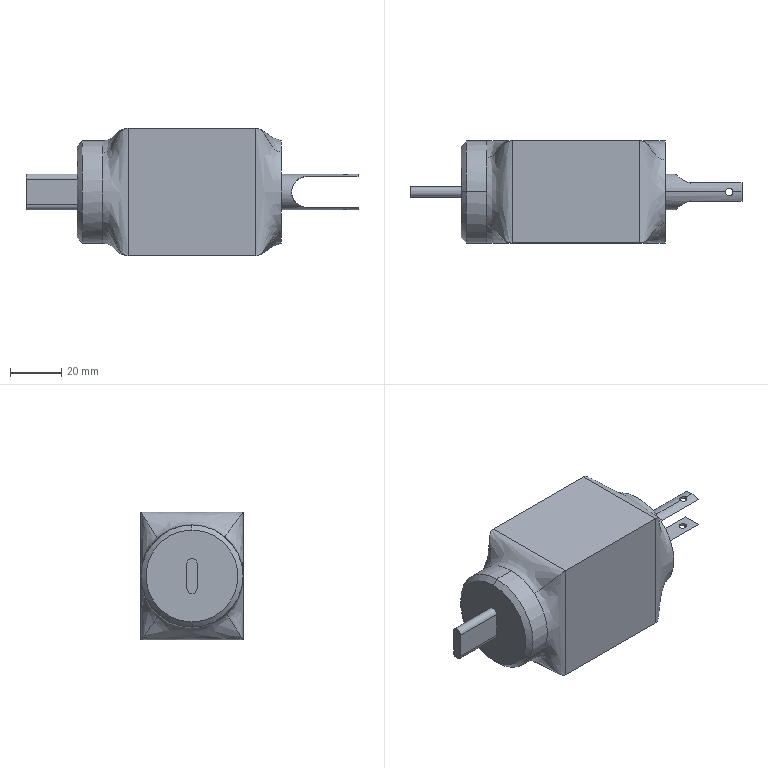Part | SolidWorks | features ICE 7, Blend 2, Chamfer 1, Extrusion 1, RefAxis 1, Revolution 1 | 1 solid | 35 faces | box 130 x 40 x 50 mm | volume 146792 mm3 | plane 13 | cylinder 12 | spline 8 | cone 2 | commonest cylinder face diameters 3 x4 4 x3 14 x2 40 x2 12 x1
STEP:
#1=CARTESIAN_POINT('',(83.5,0.,6.));
#2=VERTEX_POINT('',#1);
#3=CARTESIAN_POINT('',(86.5,0.,6.));
#4=VERTEX_POINT('',#3);
#5=CARTESIAN_POINT('',(85.,0.,6.));
#6=DIRECTION('',(0.,0.,1.));
#7=DIRECTION('',(1.,0.,0.));
#8=AXIS2_PLACEMENT_3D('',#5,#6,#7);
#9=CIRCLE('',#8,1.5);
#10=EDGE_CURVE('',#2,#4,#9,.T.);
#11=ORIENTED_EDGE('',*,*,#10,.F.);
#12=CARTESIAN_POINT('',(83.5,0.,7.));
#13=VERTEX_POINT('',#12);
#14=CARTESIAN_POINT('',(83.5,0.,-15.));
#15=DIRECTION('',(0.,0.,1.));
#16=VECTOR('',#15,1000.);
#17=LINE('',#14,#16);
#18=EDGE_CURVE('',#2,#13,#17,.T.);
#19=ORIENTED_EDGE('',*,*,#18,.T.);
#20=CARTESIAN_POINT('',(86.5,0.,7.));
#21=VERTEX_POINT('',#20);
#22=CARTESIAN_POINT('',(86.5,0.,7.));
#23=CARTESIAN_POINT('',(86.5,-0.09942,7.));
#24=CARTESIAN_POINT('',(86.49,-0.1971,6.998));
#25=CARTESIAN_POINT('',(86.452,-0.3892,6.99));
#26=CARTESIAN_POINT('',(86.423,-0.4847,6.984));
#27=CARTESIAN_POINT('',(86.348,-0.6662,6.969));
#28=CARTESIAN_POINT('',(86.301,-0.7523,6.96));
#29=CARTESIAN_POINT('',(86.193,-0.9151,6.94));
#30=CARTESIAN_POINT('',(86.129,-0.992,6.93));
#31=CARTESIAN_POINT('',(85.922,-1.199,6.898));
#32=CARTESIAN_POINT('',(85.755,-1.31,6.877));
#33=CARTESIAN_POINT('',(85.395,-1.46,6.846));
#34=CARTESIAN_POINT('',(85.197,-1.5,6.837));
#35=CARTESIAN_POINT('',(84.902,-1.5,6.837));
#36=CARTESIAN_POINT('',(84.803,-1.49,6.84));
#37=CARTESIAN_POINT('',(84.61,-1.452,6.848));
#38=CARTESIAN_POINT('',(84.516,-1.423,6.854));
#39=CARTESIAN_POINT('',(84.243,-1.31,6.877));
#40=CARTESIAN_POINT('',(84.078,-1.2,6.898));
#41=CARTESIAN_POINT('',(83.87,-0.9909,6.93));
#42=CARTESIAN_POINT('',(83.808,-0.9154,6.94));
#43=CARTESIAN_POINT('',(83.699,-0.7532,6.96));
#44=CARTESIAN_POINT('',(83.652,-0.6653,6.969));
#45=CARTESIAN_POINT('',(83.577,-0.4841,6.984));
#46=CARTESIAN_POINT('',(83.548,-0.3905,6.99));
#47=CARTESIAN_POINT('',(83.51,-0.1976,6.998));
#48=CARTESIAN_POINT('',(83.5,-0.09806,7.));
#49=CARTESIAN_POINT('',(83.5,0.,7.));
#50=B_SPLINE_CURVE_WITH_KNOTS('',3,(#22,#23,#24,#25,#26,#27,#28,#29,#30,#31,#32,#33,#34,#35,#36,#37,#38,#39,#40,#41,#42,#43,#44,#45,#46,#47,#48,#49),.UNSPECIFIED.,.F.,.F.,(4,2,2,2,2,2,2,2,2,2,2,2,2,4),(0.,0.000294,0.0005879,0.0008819,0.001176,0.001764,0.002352,0.002646,0.00294,0.003528,0.003821,0.004115,0.004409,0.004703),.UNSPECIFIED.);
#51=EDGE_CURVE('',#21,#13,#50,.T.);
#52=ORIENTED_EDGE('',*,*,#51,.F.);
#53=CARTESIAN_POINT('',(86.5,0.,-15.));
#54=DIRECTION('',(0.,0.,1.));
#55=VECTOR('',#54,1000.);
#56=LINE('',#53,#55);
#57=EDGE_CURVE('',#4,#21,#56,.T.);
#58=ORIENTED_EDGE('',*,*,#57,.F.);
#59=EDGE_LOOP('',(#11,#19,#52,#58));
#60=FACE_OUTER_BOUND('',#59,.T.);
#61=CARTESIAN_POINT('',(85.,0.,-15.));
#62=DIRECTION('',(0.,0.,1.));
#63=DIRECTION('',(1.,0.,0.));
#64=AXIS2_PLACEMENT_3D('',#61,#62,#63);
#65=CYLINDRICAL_SURFACE('',#64,1.5);
#66=ADVANCED_FACE('',(#60),#65,.F.);
#67=CARTESIAN_POINT('',(83.5,0.,-7.));
#68=VERTEX_POINT('',#67);
#69=CARTESIAN_POINT('',(86.5,0.,-7.));
#70=VERTEX_POINT('',#69);
#71=CARTESIAN_POINT('',(83.5,0.,-7.));
#72=CARTESIAN_POINT('',(83.5,-0.1961,-7.));
#73=CARTESIAN_POINT('',(83.54,-0.394,-6.991));
#74=CARTESIAN_POINT('',(83.689,-0.7552,-6.962));
#75=CARTESIAN_POINT('',(83.801,-0.9218,-6.94));
#76=CARTESIAN_POINT('',(84.008,-1.129,-6.909));
#77=CARTESIAN_POINT('',(84.085,-1.192,-6.898));
#78=CARTESIAN_POINT('',(84.247,-1.301,-6.878));
#79=CARTESIAN_POINT('',(84.333,-1.347,-6.869));
#80=CARTESIAN_POINT('',(84.606,-1.461,-6.846));
#81=CARTESIAN_POINT('',(84.801,-1.5,-6.837));
#82=CARTESIAN_POINT('',(85.098,-1.5,-6.837));
#83=CARTESIAN_POINT('',(85.196,-1.49,-6.84));
#84=CARTESIAN_POINT('',(85.388,-1.452,-6.848));
#85=CARTESIAN_POINT('',(85.484,-1.423,-6.854));
#86=CARTESIAN_POINT('',(85.756,-1.311,-6.877));
#87=CARTESIAN_POINT('',(85.922,-1.199,-6.898));
#88=CARTESIAN_POINT('',(86.198,-0.9236,-6.94));
#89=CARTESIAN_POINT('',(86.31,-0.7569,-6.961));
#90=CARTESIAN_POINT('',(86.46,-0.396,-6.991));
#91=CARTESIAN_POINT('',(86.5,-0.1988,-7.));
#92=CARTESIAN_POINT('',(86.5,0.,-7.));
#93=B_SPLINE_CURVE_WITH_KNOTS('',3,(#71,#72,#73,#74,#75,#76,#77,#78,#79,#80,#81,#82,#83,#84,#85,#86,#87,#88,#89,#90,#91,#92),.UNSPECIFIED.,.F.,.F.,(4,2,2,2,2,2,2,2,2,2,4),(0.004703,0.005291,0.005879,0.006173,0.006467,0.007054,0.007348,0.007642,0.00823,0.008818,0.009405),.UNSPECIFIED.);
#94=EDGE_CURVE('',#68,#70,#93,.T.);
#95=ORIENTED_EDGE('',*,*,#94,.F.);
#96=CARTESIAN_POINT('',(83.5,0.,-6.));
#97=VERTEX_POINT('',#96);
#98=CARTESIAN_POINT('',(83.5,0.,-15.));
#99=DIRECTION('',(0.,0.,1.));
#100=VECTOR('',#99,1000.);
#101=LINE('',#98,#100);
#102=EDGE_CURVE('',#68,#97,#101,.T.);
#103=ORIENTED_EDGE('',*,*,#102,.T.);
#104=CARTESIAN_POINT('',(86.5,0.,-6.));
#105=VERTEX_POINT('',#104);
#106=CARTESIAN_POINT('',(85.,0.,-6.));
#107=DIRECTION('',(0.,0.,-1.));
#108=DIRECTION('',(-1.,0.,0.));
#109=AXIS2_PLACEMENT_3D('',#106,#107,#108);
#110=CIRCLE('',#109,1.5);
#111=EDGE_CURVE('',#105,#97,#110,.T.);
#112=ORIENTED_EDGE('',*,*,#111,.F.);
#113=CARTESIAN_POINT('',(86.5,0.,-15.));
#114=DIRECTION('',(0.,0.,1.));
#115=VECTOR('',#114,1000.);
#116=LINE('',#113,#115);
#117=EDGE_CURVE('',#70,#105,#116,.T.);
#118=ORIENTED_EDGE('',*,*,#117,.F.);
#119=EDGE_LOOP('',(#95,#103,#112,#118));
#120=FACE_OUTER_BOUND('',#119,.T.);
#121=CARTESIAN_POINT('',(85.,0.,-15.));
#122=DIRECTION('',(0.,0.,1.));
#123=DIRECTION('',(1.,0.,0.));
#124=AXIS2_PLACEMENT_3D('',#121,#122,#123);
#125=CYLINDRICAL_SURFACE('',#124,1.5);
#126=ADVANCED_FACE('',(#120),#125,.F.);
#127=CARTESIAN_POINT('',(90.,0.,-7.));
#128=VERTEX_POINT('',#127);
#129=CARTESIAN_POINT('',(90.,3.606,-6.));
#130=VERTEX_POINT('',#129);
#131=CARTESIAN_POINT('',(90.,0.,0.));
#132=DIRECTION('',(1.,0.,0.));
#133=DIRECTION('',(0.,0.,-1.));
#134=AXIS2_PLACEMENT_3D('',#131,#132,#133);
#135=CIRCLE('',#134,7.);
#136=EDGE_CURVE('',#128,#130,#135,.T.);
#137=ORIENTED_EDGE('',*,*,#136,.F.);
#138=CARTESIAN_POINT('',(90.,0.,-7.));
#139=DIRECTION('',(-1.,0.,0.));
#140=VECTOR('',#139,1000.);
#141=LINE('',#138,#140);
#142=EDGE_CURVE('',#128,#70,#141,.T.);
#143=ORIENTED_EDGE('',*,*,#142,.T.);
#144=CARTESIAN_POINT('',(86.5,0.,-7.));
#145=CARTESIAN_POINT('',(86.5,0.09942,-7.));
#146=CARTESIAN_POINT('',(86.49,0.1971,-6.998));
#147=CARTESIAN_POINT('',(86.452,0.3892,-6.99));
#148=CARTESIAN_POINT('',(86.423,0.4847,-6.984));
#149=CARTESIAN_POINT('',(86.348,0.6662,-6.969));
#150=CARTESIAN_POINT('',(86.301,0.7523,-6.96));
#151=CARTESIAN_POINT('',(86.193,0.9151,-6.94));
#152=CARTESIAN_POINT('',(86.129,0.992,-6.93));
#153=CARTESIAN_POINT('',(85.922,1.199,-6.898));
#154=CARTESIAN_POINT('',(85.755,1.31,-6.877));
#155=CARTESIAN_POINT('',(85.395,1.46,-6.846));
#156=CARTESIAN_POINT('',(85.197,1.5,-6.837));
#157=CARTESIAN_POINT('',(84.902,1.5,-6.837));
#158=CARTESIAN_POINT('',(84.803,1.49,-6.84));
#159=CARTESIAN_POINT('',(84.61,1.452,-6.848));
#160=CARTESIAN_POINT('',(84.516,1.423,-6.854));
#161=CARTESIAN_POINT('',(84.243,1.31,-6.877));
#162=CARTESIAN_POINT('',(84.078,1.2,-6.898));
#163=CARTESIAN_POINT('',(83.87,0.9909,-6.93));
#164=CARTESIAN_POINT('',(83.808,0.9154,-6.94));
#165=CARTESIAN_POINT('',(83.699,0.7532,-6.96));
#166=CARTESIAN_POINT('',(83.652,0.6653,-6.969));
#167=CARTESIAN_POINT('',(83.577,0.4841,-6.984));
#168=CARTESIAN_POINT('',(83.548,0.3905,-6.99));
#169=CARTESIAN_POINT('',(83.51,0.1976,-6.998));
#170=CARTESIAN_POINT('',(83.5,0.09806,-7.));
#171=CARTESIAN_POINT('',(83.5,0.,-7.));
#172=B_SPLINE_CURVE_WITH_KNOTS('',3,(#144,#145,#146,#147,#148,#149,#150,#151,#152,#153,#154,#155,#156,#157,#158,#159,#160,#161,#162,#163,#164,#165,#166,#167,#168,#169,#170,#171),.UNSPECIFIED.,.F.,.F.,(4,2,2,2,2,2,2,2,2,2,2,2,2,4),(0.,0.000294,0.0005879,0.0008819,0.001176,0.001764,0.002352,0.002646,0.00294,0.003528,0.003821,0.004115,0.004409,0.004703),.UNSPECIFIED.);
#173=EDGE_CURVE('',#70,#68,#172,.T.);
#174=ORIENTED_EDGE('',*,*,#173,.T.);
#175=CARTESIAN_POINT('',(60.,0.,-7.));
#176=VERTEX_POINT('',#175);
#177=CARTESIAN_POINT('',(90.,0.,-7.));
#178=DIRECTION('',(-1.,0.,0.));
#179=VECTOR('',#178,1000.);
#180=LINE('',#177,#179);
#181=EDGE_CURVE('',#68,#176,#180,.T.);
#182=ORIENTED_EDGE('',*,*,#181,.T.);
#183=CARTESIAN_POINT('',(60.,0.,7.));
#184=VERTEX_POINT('',#183);
#185=CARTESIAN_POINT('',(60.,0.,0.));
#186=DIRECTION('',(1.,0.,0.));
#187=DIRECTION('',(0.,0.,-1.));
#188=AXIS2_PLACEMENT_3D('',#185,#186,#187);
#189=CIRCLE('',#188,7.);
#190=EDGE_CURVE('',#176,#184,#189,.T.);
#191=ORIENTED_EDGE('',*,*,#190,.T.);
#192=CARTESIAN_POINT('',(90.,0.,7.));
#193=DIRECTION('',(-1.,0.,0.));
#194=VECTOR('',#193,1000.);
#195=LINE('',#192,#194);
#196=EDGE_CURVE('',#13,#184,#195,.T.);
#197=ORIENTED_EDGE('',*,*,#196,.F.);
#198=CARTESIAN_POINT('',(83.5,0.,7.));
#199=CARTESIAN_POINT('',(83.5,0.1961,7.));
#200=CARTESIAN_POINT('',(83.54,0.394,6.991));
#201=CARTESIAN_POINT('',(83.689,0.7552,6.962));
#202=CARTESIAN_POINT('',(83.801,0.9218,6.94));
#203=CARTESIAN_POINT('',(84.008,1.129,6.909));
#204=CARTESIAN_POINT('',(84.085,1.192,6.898));
#205=CARTESIAN_POINT('',(84.247,1.301,6.878));
#206=CARTESIAN_POINT('',(84.333,1.347,6.869));
#207=CARTESIAN_POINT('',(84.606,1.461,6.846));
#208=CARTESIAN_POINT('',(84.801,1.5,6.837));
#209=CARTESIAN_POINT('',(85.098,1.5,6.837));
#210=CARTESIAN_POINT('',(85.196,1.49,6.84));
#211=CARTESIAN_POINT('',(85.388,1.452,6.848));
#212=CARTESIAN_POINT('',(85.484,1.423,6.854));
#213=CARTESIAN_POINT('',(85.756,1.311,6.877));
#214=CARTESIAN_POINT('',(85.922,1.199,6.898));
#215=CARTESIAN_POINT('',(86.198,0.9236,6.94));
#216=CARTESIAN_POINT('',(86.31,0.7569,6.961));
#217=CARTESIAN_POINT('',(86.46,0.396,6.991));
#218=CARTESIAN_POINT('',(86.5,0.1988,7.));
#219=CARTESIAN_POINT('',(86.5,0.,7.));
#220=B_SPLINE_CURVE_WITH_KNOTS('',3,(#198,#199,#200,#201,#202,#203,#204,#205,#206,#207,#208,#209,#210,#211,#212,#213,#214,#215,#216,#217,#218,#219),.UNSPECIFIED.,.F.,.F.,(4,2,2,2,2,2,2,2,2,2,4),(0.004703,0.005291,0.005879,0.006173,0.006467,0.007054,0.007348,0.007642,0.00823,0.008818,0.009405),.UNSPECIFIED.);
#221=EDGE_CURVE('',#13,#21,#220,.T.);
#222=ORIENTED_EDGE('',*,*,#221,.T.);
#223=CARTESIAN_POINT('',(90.,0.,7.));
#224=VERTEX_POINT('',#223);
#225=CARTESIAN_POINT('',(90.,0.,7.));
#226=DIRECTION('',(-1.,0.,0.));
#227=VECTOR('',#226,1000.);
#228=LINE('',#225,#227);
#229=EDGE_CURVE('',#224,#21,#228,.T.);
#230=ORIENTED_EDGE('',*,*,#229,.F.);
#231=CARTESIAN_POINT('',(90.,3.606,6.));
#232=VERTEX_POINT('',#231);
#233=CARTESIAN_POINT('',(90.,0.,0.));
#234=DIRECTION('',(1.,0.,0.));
#235=DIRECTION('',(0.,0.,-1.));
#236=AXIS2_PLACEMENT_3D('',#233,#234,#235);
#237=CIRCLE('',#236,7.);
#238=EDGE_CURVE('',#232,#224,#237,.T.);
#239=ORIENTED_EDGE('',*,*,#238,.F.);
#240=CARTESIAN_POINT('',(70.,3.606,6.));
#241=VERTEX_POINT('',#240);
#242=CARTESIAN_POINT('',(90.,3.606,6.));
#243=DIRECTION('',(-1.,0.,0.));
#244=VECTOR('',#243,1000.);
#245=LINE('',#242,#244);
#246=EDGE_CURVE('',#232,#241,#245,.T.);
#247=ORIENTED_EDGE('',*,*,#246,.T.);
#248=CARTESIAN_POINT('',(70.,3.606,-6.));
#249=VERTEX_POINT('',#248);
#250=CARTESIAN_POINT('',(70.,3.606,6.));
#251=CARTESIAN_POINT('',(69.572,3.606,6.));
#252=CARTESIAN_POINT('',(69.158,3.683,5.955));
#253=CARTESIAN_POINT('',(68.364,3.942,5.787));
#254=CARTESIAN_POINT('',(67.998,4.114,5.669));
#255=CARTESIAN_POINT('',(67.477,4.398,5.447));
#256=CARTESIAN_POINT('',(67.308,4.498,5.365));
#257=CARTESIAN_POINT('',(66.981,4.701,5.189));
#258=CARTESIAN_POINT('',(66.824,4.804,5.094));
#259=CARTESIAN_POINT('',(66.368,5.113,4.79));
#260=CARTESIAN_POINT('',(66.084,5.32,4.561));
#261=CARTESIAN_POINT('',(65.553,5.722,4.045));
#262=CARTESIAN_POINT('',(65.306,5.918,3.756));
#263=CARTESIAN_POINT('',(64.867,6.271,3.131));
#264=CARTESIAN_POINT('',(64.674,6.431,2.793));
#265=CARTESIAN_POINT('',(64.348,6.703,2.054));
#266=CARTESIAN_POINT('',(64.221,6.811,1.667));
#267=CARTESIAN_POINT('',(64.09,6.923,1.058));
#268=CARTESIAN_POINT('',(64.057,6.952,0.8481));
#269=CARTESIAN_POINT('',(64.012,6.99,0.4287));
#270=CARTESIAN_POINT('',(63.989,7.009,0.009133));
#271=CARTESIAN_POINT('',(64.01,6.991,-0.4109));
#272=CARTESIAN_POINT('',(64.054,6.954,-0.831));
#273=CARTESIAN_POINT('',(64.087,6.925,-1.041));
#274=CARTESIAN_POINT('',(64.174,6.852,-1.448));
#275=CARTESIAN_POINT('',(64.227,6.807,-1.646));
#276=CARTESIAN_POINT('',(64.352,6.701,-2.035));
#277=CARTESIAN_POINT('',(64.425,6.639,-2.227));
#278=CARTESIAN_POINT('',(64.667,6.436,-2.78));
#279=CARTESIAN_POINT('',(64.86,6.277,-3.119));
#280=CARTESIAN_POINT('',(65.191,6.01,-3.593));
#281=CARTESIAN_POINT('',(65.308,5.917,-3.745));
#282=CARTESIAN_POINT('',(65.552,5.725,-4.031));
#283=CARTESIAN_POINT('',(65.679,5.627,-4.167));
#284=CARTESIAN_POINT('',(66.075,5.327,-4.553));
#285=CARTESIAN_POINT('',(66.359,5.119,-4.783));
#286=CARTESIAN_POINT('',(66.972,4.703,-5.193));
#287=CARTESIAN_POINT('',(67.298,4.496,-5.371));
#288=CARTESIAN_POINT('',(67.817,4.212,-5.592));
#289=CARTESIAN_POINT('',(67.996,4.122,-5.659));
#290=CARTESIAN_POINT('',(68.366,3.955,-5.777));
#291=CARTESIAN_POINT('',(68.56,3.878,-5.828));
#292=CARTESIAN_POINT('',(68.954,3.75,-5.912));
#293=CARTESIAN_POINT('',(69.156,3.697,-5.944));
#294=CARTESIAN_POINT('',(69.572,3.625,-5.988));
#295=CARTESIAN_POINT('',(69.786,3.606,-6.));
#296=CARTESIAN_POINT('',(70.,3.606,-6.));
#297=B_SPLINE_CURVE_WITH_KNOTS('',3,(#250,#251,#252,#253,#254,#255,#256,#257,#258,#259,#260,#261,#262,#263,#264,#265,#266,#267,#268,#269,#270,#271,#272,#273,#274,#275,#276,#277,#278,#279,#280,#281,#282,#283,#284,#285,#286,#287,#288,#289,#290,#291,#292,#293,#294,#295,#296),.UNSPECIFIED.,.F.,.F.,(4,2,2,2,2,2,2,2,2,2,1,2,2,2,2,2,2,2,2,2,2,2,2,4),(0.,0.001263,0.002526,0.003157,0.003789,0.005052,0.006315,0.007578,0.008841,0.009472,0.0101,0.01073,0.01137,0.012,0.01263,0.01389,0.01452,0.01516,0.01642,0.01768,0.01831,0.01894,0.01958,0.02021),.UNSPECIFIED.);
#298=EDGE_CURVE('',#241,#249,#297,.T.);
#299=ORIENTED_EDGE('',*,*,#298,.T.);
#300=CARTESIAN_POINT('',(90.,3.606,-6.));
#301=DIRECTION('',(1.,0.,0.));
#302=VECTOR('',#301,1000.);
#303=LINE('',#300,#302);
#304=EDGE_CURVE('',#249,#130,#303,.T.);
#305=ORIENTED_EDGE('',*,*,#304,.T.);
#306=EDGE_LOOP('',(#137,#143,#174,#182,#191,#197,#222,#230,#239,#247,#299,#305));
#307=FACE_OUTER_BOUND('',#306,.T.);
#308=CARTESIAN_POINT('',(90.,0.,0.));
#309=DIRECTION('',(-1.,0.,0.));
#310=DIRECTION('',(0.,0.,1.));
#311=AXIS2_PLACEMENT_3D('',#308,#309,#310);
#312=CYLINDRICAL_SURFACE('',#311,7.);
#313=ADVANCED_FACE('',(#307),#312,.T.);
#314=CARTESIAN_POINT('',(-40.,0.,-7.));
#315=VERTEX_POINT('',#314);
#316=CARTESIAN_POINT('',(-40.,-2.,-5.));
#317=VERTEX_POINT('',#316);
#318=CARTESIAN_POINT('',(-40.,0.,-5.));
#319=DIRECTION('',(-1.,0.,0.));
#320=DIRECTION('',(0.,0.,1.));
#321=AXIS2_PLACEMENT_3D('',#318,#319,#320);
#322=CIRCLE('',#321,2.);
#323=EDGE_CURVE('',#315,#317,#322,.T.);
#324=ORIENTED_EDGE('',*,*,#323,.F.);
#325=CARTESIAN_POINT('',(-20.,0.,-7.));
#326=VERTEX_POINT('',#325);
#327=CARTESIAN_POINT('',(-40.,0.,-7.));
#328=DIRECTION('',(1.,0.,0.));
#329=VECTOR('',#328,1000.);
#330=LINE('',#327,#329);
#331=EDGE_CURVE('',#315,#326,#330,.T.);
#332=ORIENTED_EDGE('',*,*,#331,.T.);
#333=CARTESIAN_POINT('',(-20.,-2.,-5.));
#334=VERTEX_POINT('',#333);
#335=CARTESIAN_POINT('',(-20.,0.,-5.));
#336=DIRECTION('',(-1.,0.,0.));
#337=DIRECTION('',(0.,0.,1.));
#338=AXIS2_PLACEMENT_3D('',#335,#336,#337);
#339=CIRCLE('',#338,2.);
#340=EDGE_CURVE('',#326,#334,#339,.T.);
#341=ORIENTED_EDGE('',*,*,#340,.T.);
#342=CARTESIAN_POINT('',(-40.,-2.,-5.));
#343=DIRECTION('',(1.,0.,0.));
#344=VECTOR('',#343,1000.);
#345=LINE('',#342,#344);
#346=EDGE_CURVE('',#317,#334,#345,.T.);
#347=ORIENTED_EDGE('',*,*,#346,.F.);
#348=EDGE_LOOP('',(#324,#332,#341,#347));
#349=FACE_OUTER_BOUND('',#348,.T.);
#350=CARTESIAN_POINT('',(-40.,0.,-5.));
#351=DIRECTION('',(1.,0.,0.));
#352=DIRECTION('',(0.,0.,-1.));
#353=AXIS2_PLACEMENT_3D('',#350,#351,#352);
#354=CYLINDRICAL_SURFACE('',#353,2.);
#355=ADVANCED_FACE('',(#349),#354,.T.);
#356=CARTESIAN_POINT('',(-20.,0.,18.));
#357=VERTEX_POINT('',#356);
#358=CARTESIAN_POINT('',(-20.,0.,-18.));
#359=VERTEX_POINT('',#358);
#360=CARTESIAN_POINT('',(-20.,0.,0.));
#361=DIRECTION('',(-1.,0.,0.));
#362=DIRECTION('',(0.,0.,1.));
#363=AXIS2_PLACEMENT_3D('',#360,#361,#362);
#364=CIRCLE('',#363,18.);
#365=EDGE_CURVE('',#357,#359,#364,.T.);
#366=ORIENTED_EDGE('',*,*,#365,.F.);
#367=CARTESIAN_POINT('',(-18.,0.,20.));
#368=VERTEX_POINT('',#367);
#369=CARTESIAN_POINT('',(-20.,0.,18.));
#370=DIRECTION('',(0.7071,0.,0.7071));
#371=VECTOR('',#370,1000.);
#372=LINE('',#369,#371);
#373=EDGE_CURVE('',#357,#368,#372,.T.);
#374=ORIENTED_EDGE('',*,*,#373,.T.);
#375=CARTESIAN_POINT('',(-18.,0.,-20.));
#376=VERTEX_POINT('',#375);
#377=CARTESIAN_POINT('',(-18.,0.,0.));
#378=DIRECTION('',(1.,0.,0.));
#379=DIRECTION('',(0.,0.,1.));
#380=AXIS2_PLACEMENT_3D('',#377,#378,#379);
#381=CIRCLE('',#380,20.);
#382=EDGE_CURVE('',#376,#368,#381,.T.);
#383=ORIENTED_EDGE('',*,*,#382,.F.);
#384=CARTESIAN_POINT('',(-20.,0.,-18.));
#385=DIRECTION('',(0.7071,0.,-0.7071));
#386=VECTOR('',#385,1000.);
#387=LINE('',#384,#386);
#388=EDGE_CURVE('',#359,#376,#387,.T.);
#389=ORIENTED_EDGE('',*,*,#388,.F.);
#390=EDGE_LOOP('',(#366,#374,#383,#389));
#391=FACE_OUTER_BOUND('',#390,.T.);
#392=CARTESIAN_POINT('',(-20.,0.,0.));
#393=DIRECTION('',(1.,0.,0.));
#394=DIRECTION('',(0.,0.,-1.));
#395=AXIS2_PLACEMENT_3D('',#392,#393,#394);
#396=CONICAL_SURFACE('',#395,18.,0.7854);
#397=ADVANCED_FACE('',(#391),#396,.T.);
#398=ORIENTED_EDGE('',*,*,#382,.T.);
#399=CARTESIAN_POINT('',(-10.,-0.000000219,19.999));
#400=VERTEX_POINT('',#399);
#401=CARTESIAN_POINT('',(-20.,0.,20.));
#402=DIRECTION('',(1.,0.,0.));
#403=VECTOR('',#402,1000.);
#404=LINE('',#401,#403);
#405=EDGE_CURVE('',#368,#400,#404,.T.);
#406=ORIENTED_EDGE('',*,*,#405,.T.);
#407=CARTESIAN_POINT('',(-10.,13.524,14.735));
#408=VERTEX_POINT('',#407);
#409=CARTESIAN_POINT('',(-10.,0.,0.));
#410=DIRECTION('',(-1.,0.,0.));
#411=DIRECTION('',(0.,0.,1.));
#412=AXIS2_PLACEMENT_3D('',#409,#410,#411);
#413=CIRCLE('',#412,20.);
#414=EDGE_CURVE('',#400,#408,#413,.T.);
#415=ORIENTED_EDGE('',*,*,#414,.T.);
#416=CARTESIAN_POINT('',(-10.,12.81,-15.361));
#417=VERTEX_POINT('',#416);
#418=CARTESIAN_POINT('',(-10.,0.,0.));
#419=DIRECTION('',(-1.,0.,0.));
#420=DIRECTION('',(0.,0.,1.));
#421=AXIS2_PLACEMENT_3D('',#418,#419,#420);
#422=CIRCLE('',#421,20.);
#423=EDGE_CURVE('',#408,#417,#422,.T.);
#424=ORIENTED_EDGE('',*,*,#423,.T.);
#425=CARTESIAN_POINT('',(-10.,0.000000292,-19.999));
#426=VERTEX_POINT('',#425);
#427=CARTESIAN_POINT('',(-10.,0.,0.));
#428=DIRECTION('',(-1.,0.,0.));
#429=DIRECTION('',(0.,0.,1.));
#430=AXIS2_PLACEMENT_3D('',#427,#428,#429);
#431=CIRCLE('',#430,20.);
#432=EDGE_CURVE('',#417,#426,#431,.T.);
#433=ORIENTED_EDGE('',*,*,#432,.T.);
#434=CARTESIAN_POINT('',(-20.,0.,-20.));
#435=DIRECTION('',(1.,0.,0.));
#436=VECTOR('',#435,1000.);
#437=LINE('',#434,#436);
#438=EDGE_CURVE('',#376,#426,#437,.T.);
#439=ORIENTED_EDGE('',*,*,#438,.F.);
#440=EDGE_LOOP('',(#398,#406,#415,#424,#433,#439));
#441=FACE_OUTER_BOUND('',#440,.T.);
#442=CARTESIAN_POINT('',(-20.,0.,0.));
#443=DIRECTION('',(1.,0.,0.));
#444=DIRECTION('',(0.,0.,-1.));
#445=AXIS2_PLACEMENT_3D('',#442,#443,#444);
#446=CYLINDRICAL_SURFACE('',#445,20.);
#447=ADVANCED_FACE('',(#441),#446,.T.);
#448=CARTESIAN_POINT('',(90.,-3.606,6.));
#449=VERTEX_POINT('',#448);
#450=CARTESIAN_POINT('',(90.,0.,6.));
#451=DIRECTION('',(0.,-1.,0.));
#452=VECTOR('',#451,1000.);
#453=LINE('',#450,#452);
#454=EDGE_CURVE('',#232,#449,#453,.T.);
#455=ORIENTED_EDGE('',*,*,#454,.F.);
#456=ORIENTED_EDGE('',*,*,#238,.T.);
#457=CARTESIAN_POINT('',(90.,0.,0.));
#458=DIRECTION('',(1.,0.,0.));
#459=DIRECTION('',(0.,0.,-1.));
#460=AXIS2_PLACEMENT_3D('',#457,#458,#459);
#461=CIRCLE('',#460,7.);
#462=EDGE_CURVE('',#224,#449,#461,.T.);
#463=ORIENTED_EDGE('',*,*,#462,.T.);
#464=EDGE_LOOP('',(#455,#456,#463));
#465=FACE_OUTER_BOUND('',#464,.T.);
#466=CARTESIAN_POINT('',(90.,0.,0.));
#467=DIRECTION('',(1.,0.,0.));
#468=DIRECTION('',(0.,0.,-1.));
#469=AXIS2_PLACEMENT_3D('',#466,#467,#468);
#470=PLANE('',#469);
#471=ADVANCED_FACE('',(#465),#470,.T.);
#472=CARTESIAN_POINT('',(60.,-12.494,-15.617));
#473=VERTEX_POINT('',#472);
#474=CARTESIAN_POINT('',(60.,12.494,-15.617));
#475=VERTEX_POINT('',#474);
#476=CARTESIAN_POINT('',(60.,0.,0.));
#477=DIRECTION('',(1.,0.,0.));
#478=DIRECTION('',(0.,0.,-1.));
#479=AXIS2_PLACEMENT_3D('',#476,#477,#478);
#480=CIRCLE('',#479,20.);
#481=EDGE_CURVE('',#473,#475,#480,.T.);
#482=ORIENTED_EDGE('',*,*,#481,.T.);
#483=CARTESIAN_POINT('',(60.,12.494,15.617));
#484=VERTEX_POINT('',#483);
#485=CARTESIAN_POINT('',(60.,0.,0.));
#486=DIRECTION('',(1.,0.,0.));
#487=DIRECTION('',(0.,0.,-1.));
#488=AXIS2_PLACEMENT_3D('',#485,#486,#487);
#489=CIRCLE('',#488,20.);
#490=EDGE_CURVE('',#475,#484,#489,.T.);
#491=ORIENTED_EDGE('',*,*,#490,.T.);
#492=CARTESIAN_POINT('',(60.,-12.494,15.617));
#493=VERTEX_POINT('',#492);
#494=CARTESIAN_POINT('',(60.,0.,0.));
#495=DIRECTION('',(1.,0.,0.));
#496=DIRECTION('',(0.,0.,-1.));
#497=AXIS2_PLACEMENT_3D('',#494,#495,#496);
#498=CIRCLE('',#497,20.);
#499=EDGE_CURVE('',#484,#493,#498,.T.);
#500=ORIENTED_EDGE('',*,*,#499,.T.);
#501=CARTESIAN_POINT('',(60.,0.,0.));
#502=DIRECTION('',(1.,0.,0.));
#503=DIRECTION('',(0.,0.,-1.));
#504=AXIS2_PLACEMENT_3D('',#501,#502,#503);
#505=CIRCLE('',#504,20.);
#506=EDGE_CURVE('',#493,#473,#505,.T.);
#507=ORIENTED_EDGE('',*,*,#506,.T.);
#508=EDGE_LOOP('',(#482,#491,#500,#507));
#509=FACE_OUTER_BOUND('',#508,.T.);
#510=CARTESIAN_POINT('',(60.,0.,0.));
#511=DIRECTION('',(1.,0.,0.));
#512=DIRECTION('',(0.,0.,-1.));
#513=AXIS2_PLACEMENT_3D('',#510,#511,#512);
#514=CIRCLE('',#513,7.);
#515=EDGE_CURVE('',#184,#176,#514,.T.);
#516=ORIENTED_EDGE('',*,*,#515,.F.);
#517=ORIENTED_EDGE('',*,*,#190,.F.);
#518=EDGE_LOOP('',(#516,#517));
#519=FACE_BOUND('',#518,.T.);
#520=CARTESIAN_POINT('',(60.,0.,0.));
#521=DIRECTION('',(1.,0.,0.));
#522=DIRECTION('',(0.,0.,-1.));
#523=AXIS2_PLACEMENT_3D('',#520,#521,#522);
#524=PLANE('',#523);
#525=ADVANCED_FACE('',(#509,#519),#524,.T.);
#526=CARTESIAN_POINT('',(-20.,0.,0.));
#527=DIRECTION('',(-1.,0.,0.));
#528=DIRECTION('',(0.,0.,1.));
#529=AXIS2_PLACEMENT_3D('',#526,#527,#528);
#530=CIRCLE('',#529,18.);
#531=EDGE_CURVE('',#359,#357,#530,.T.);
#532=ORIENTED_EDGE('',*,*,#531,.T.);
#533=ORIENTED_EDGE('',*,*,#365,.T.);
#534=EDGE_LOOP('',(#532,#533));
#535=FACE_OUTER_BOUND('',#534,.T.);
#536=CARTESIAN_POINT('',(-20.,-2.,5.));
#537=VERTEX_POINT('',#536);
#538=CARTESIAN_POINT('',(-20.,-2.,-5.));
#539=DIRECTION('',(0.,0.,1.));
#540=VECTOR('',#539,1000.);
#541=LINE('',#538,#540);
#542=EDGE_CURVE('',#334,#537,#541,.T.);
#543=ORIENTED_EDGE('',*,*,#542,.F.);
#544=ORIENTED_EDGE('',*,*,#340,.F.);
#545=CARTESIAN_POINT('',(-20.,2.,-5.));
#546=VERTEX_POINT('',#545);
#547=CARTESIAN_POINT('',(-20.,0.,-5.));
#548=DIRECTION('',(-1.,0.,0.));
#549=DIRECTION('',(0.,0.,1.));
#550=AXIS2_PLACEMENT_3D('',#547,#548,#549);
#551=CIRCLE('',#550,2.);
#552=EDGE_CURVE('',#546,#326,#551,.T.);
#553=ORIENTED_EDGE('',*,*,#552,.F.);
#554=CARTESIAN_POINT('',(-20.,2.,5.));
#555=VERTEX_POINT('',#554);
#556=CARTESIAN_POINT('',(-20.,2.,-5.));
#557=DIRECTION('',(0.,0.,-1.));
#558=VECTOR('',#557,1000.);
#559=LINE('',#556,#558);
#560=EDGE_CURVE('',#555,#546,#559,.T.);
#561=ORIENTED_EDGE('',*,*,#560,.F.);
#562=CARTESIAN_POINT('',(-20.,0.,5.));
#563=DIRECTION('',(-1.,0.,0.));
#564=DIRECTION('',(0.,0.,1.));
#565=AXIS2_PLACEMENT_3D('',#562,#563,#564);
#566=CIRCLE('',#565,2.);
#567=EDGE_CURVE('',#537,#555,#566,.T.);
#568=ORIENTED_EDGE('',*,*,#567,.F.);
#569=EDGE_LOOP('',(#543,#544,#553,#561,#568));
#570=FACE_BOUND('',#569,.T.);
#571=CARTESIAN_POINT('',(-20.,0.,0.));
#572=DIRECTION('',(-1.,0.,0.));
#573=DIRECTION('',(0.,0.,1.));
#574=AXIS2_PLACEMENT_3D('',#571,#572,#573);
#575=PLANE('',#574);
#576=ADVANCED_FACE('',(#535,#570),#575,.T.);
#577=CARTESIAN_POINT('',(0.,-20.,-25.));
#578=VERTEX_POINT('',#577);
#579=CARTESIAN_POINT('',(0.,20.,-25.));
#580=VERTEX_POINT('',#579);
#581=CARTESIAN_POINT('',(0.,20.,-25.));
#582=DIRECTION('',(0.,1.,0.));
#583=VECTOR('',#582,1000.);
#584=LINE('',#581,#583);
#585=EDGE_CURVE('',#578,#580,#584,.T.);
#586=ORIENTED_EDGE('',*,*,#585,.T.);
#587=CARTESIAN_POINT('',(50.,20.,-25.));
#588=VERTEX_POINT('',#587);
#589=CARTESIAN_POINT('',(50.,20.,-25.));
#590=DIRECTION('',(-1.,0.,0.));
#591=VECTOR('',#590,1000.);
#592=LINE('',#589,#591);
#593=EDGE_CURVE('',#588,#580,#592,.T.);
#594=ORIENTED_EDGE('',*,*,#593,.F.);
#595=CARTESIAN_POINT('',(50.,-20.,-25.));
#596=VERTEX_POINT('',#595);
#597=CARTESIAN_POINT('',(50.,20.,-25.));
#598=DIRECTION('',(0.,1.,0.));
#599=VECTOR('',#598,1000.);
#600=LINE('',#597,#599);
#601=EDGE_CURVE('',#596,#588,#600,.T.);
#602=ORIENTED_EDGE('',*,*,#601,.F.);
#603=CARTESIAN_POINT('',(50.,-20.,-25.));
#604=DIRECTION('',(-1.,0.,0.));
#605=VECTOR('',#604,1000.);
#606=LINE('',#603,#605);
#607=EDGE_CURVE('',#596,#578,#606,.T.);
#608=ORIENTED_EDGE('',*,*,#607,.T.);
#609=EDGE_LOOP('',(#586,#594,#602,#608));
#610=FACE_OUTER_BOUND('',#609,.T.);
#611=CARTESIAN_POINT('',(50.,20.,-25.));
#612=DIRECTION('',(0.,0.,1.));
#613=DIRECTION('',(0.,-1.,0.));
#614=AXIS2_PLACEMENT_3D('',#611,#612,#613);
#615=PLANE('',#614);
#616=ADVANCED_FACE('',(#610),#615,.F.);
#617=CARTESIAN_POINT('',(0.,20.,25.));
#618=VERTEX_POINT('',#617);
#619=CARTESIAN_POINT('',(0.,20.,25.));
#620=DIRECTION('',(0.,0.,1.));
#621=VECTOR('',#620,1000.);
#622=LINE('',#619,#621);
#623=EDGE_CURVE('',#580,#618,#622,.T.);
#624=ORIENTED_EDGE('',*,*,#623,.T.);
#625=CARTESIAN_POINT('',(50.,20.,25.));
#626=VERTEX_POINT('',#625);
#627=CARTESIAN_POINT('',(50.,20.,25.));
#628=DIRECTION('',(-1.,0.,0.));
#629=VECTOR('',#628,1000.);
#630=LINE('',#627,#629);
#631=EDGE_CURVE('',#626,#618,#630,.T.);
#632=ORIENTED_EDGE('',*,*,#631,.F.);
#633=CARTESIAN_POINT('',(50.,20.,25.));
#634=DIRECTION('',(0.,0.,1.));
#635=VECTOR('',#634,1000.);
#636=LINE('',#633,#635);
#637=EDGE_CURVE('',#588,#626,#636,.T.);
#638=ORIENTED_EDGE('',*,*,#637,.F.);
#639=ORIENTED_EDGE('',*,*,#593,.T.);
#640=EDGE_LOOP('',(#624,#632,#638,#639));
#641=FACE_OUTER_BOUND('',#640,.T.);
#642=CARTESIAN_POINT('',(50.,20.,25.));
#643=DIRECTION('',(0.,-1.,0.));
#644=DIRECTION('',(0.,0.,-1.));
#645=AXIS2_PLACEMENT_3D('',#642,#643,#644);
#646=PLANE('',#645);
#647=ADVANCED_FACE('',(#641),#646,.F.);
#648=CARTESIAN_POINT('',(0.,-20.,25.));
#649=VERTEX_POINT('',#648);
#650=CARTESIAN_POINT('',(0.,20.,25.));
#651=DIRECTION('',(0.,-1.,0.));
#652=VECTOR('',#651,1000.);
#653=LINE('',#650,#652);
#654=EDGE_CURVE('',#618,#649,#653,.T.);
#655=ORIENTED_EDGE('',*,*,#654,.T.);
#656=CARTESIAN_POINT('',(50.,-20.,25.));
#657=VERTEX_POINT('',#656);
#658=CARTESIAN_POINT('',(50.,-20.,25.));
#659=DIRECTION('',(-1.,0.,0.));
#660=VECTOR('',#659,1000.);
#661=LINE('',#658,#660);
#662=EDGE_CURVE('',#657,#649,#661,.T.);
#663=ORIENTED_EDGE('',*,*,#662,.F.);
#664=CARTESIAN_POINT('',(50.,20.,25.));
#665=DIRECTION('',(0.,-1.,0.));
#666=VECTOR('',#665,1000.);
#667=LINE('',#664,#666);
#668=EDGE_CURVE('',#626,#657,#667,.T.);
#669=ORIENTED_EDGE('',*,*,#668,.F.);
#670=ORIENTED_EDGE('',*,*,#631,.T.);
#671=EDGE_LOOP('',(#655,#663,#669,#670));
#672=FACE_OUTER_BOUND('',#671,.T.);
#673=CARTESIAN_POINT('',(50.,20.,25.));
#674=DIRECTION('',(0.,0.,-1.));
#675=DIRECTION('',(-1.,0.,0.));
#676=AXIS2_PLACEMENT_3D('',#673,#674,#675);
#677=PLANE('',#676);
#678=ADVANCED_FACE('',(#672),#677,.F.);
#679=CARTESIAN_POINT('',(0.,-20.,25.));
#680=DIRECTION('',(0.,0.,-1.));
#681=VECTOR('',#680,1000.);
#682=LINE('',#679,#681);
#683=EDGE_CURVE('',#649,#578,#682,.T.);
#684=ORIENTED_EDGE('',*,*,#683,.T.);
#685=ORIENTED_EDGE('',*,*,#607,.F.);
#686=CARTESIAN_POINT('',(50.,-20.,25.));
#687=DIRECTION('',(0.,0.,-1.));
#688=VECTOR('',#687,1000.);
#689=LINE('',#686,#688);
#690=EDGE_CURVE('',#657,#596,#689,.T.);
#691=ORIENTED_EDGE('',*,*,#690,.F.);
#692=ORIENTED_EDGE('',*,*,#662,.T.);
#693=EDGE_LOOP('',(#684,#685,#691,#692));
#694=FACE_OUTER_BOUND('',#693,.T.);
#695=CARTESIAN_POINT('',(50.,-20.,25.));
#696=DIRECTION('',(0.,1.,0.));
#697=DIRECTION('',(0.,0.,1.));
#698=AXIS2_PLACEMENT_3D('',#695,#696,#697);
#699=PLANE('',#698);
#700=ADVANCED_FACE('',(#694),#699,.F.);
#701=ORIENTED_EDGE('',*,*,#423,.F.);
#702=CARTESIAN_POINT('',(-10.,13.524,14.735));
#703=CARTESIAN_POINT('',(-4.758,13.524,14.735));
#704=CARTESIAN_POINT('',(-5.242,20.,25.));
#705=CARTESIAN_POINT('',(0.,20.,25.));
#706=B_SPLINE_CURVE_WITH_KNOTS('',3,(#702,#703,#704,#705),.UNSPECIFIED.,.F.,.F.,(4,4),(0.,1.),.UNSPECIFIED.);
#707=EDGE_CURVE('',#408,#618,#706,.T.);
#708=ORIENTED_EDGE('',*,*,#707,.T.);
#709=ORIENTED_EDGE('',*,*,#623,.F.);
#710=CARTESIAN_POINT('',(0.,20.,-25.));
#711=CARTESIAN_POINT('',(-5.214,20.,-25.));
#712=CARTESIAN_POINT('',(-4.786,12.809,-15.36));
#713=CARTESIAN_POINT('',(-10.,12.81,-15.361));
#714=B_SPLINE_CURVE_WITH_KNOTS('',3,(#710,#711,#712,#713),.UNSPECIFIED.,.F.,.F.,(4,4),(0.,1.),.UNSPECIFIED.);
#715=EDGE_CURVE('',#580,#417,#714,.T.);
#716=ORIENTED_EDGE('',*,*,#715,.T.);
#717=EDGE_LOOP('',(#701,#708,#709,#716));
#718=FACE_OUTER_BOUND('',#717,.T.);
#719=CARTESIAN_POINT('',(-10.,12.809,-15.36));
#720=CARTESIAN_POINT('',(-4.786,12.809,-15.36));
#721=CARTESIAN_POINT('',(-5.214,20.,-25.));
#722=CARTESIAN_POINT('',(0.,20.,-25.));
#723=CARTESIAN_POINT('',(-10.,17.238,-11.666));
#724=CARTESIAN_POINT('',(-5.727,17.238,-11.666));
#725=CARTESIAN_POINT('',(-4.273,20.,-16.667));
#726=CARTESIAN_POINT('',(0.,20.,-16.667));
#727=CARTESIAN_POINT('',(-10.,19.858,-6.24));
#728=CARTESIAN_POINT('',(-6.668,19.858,-6.24));
#729=CARTESIAN_POINT('',(-3.332,20.,-8.333));
#730=CARTESIAN_POINT('',(0.,20.,-8.333));
#731=CARTESIAN_POINT('',(-10.,20.131,5.291));
#732=CARTESIAN_POINT('',(-6.658,20.131,5.291));
#733=CARTESIAN_POINT('',(-3.342,20.,8.333));
#734=CARTESIAN_POINT('',(0.,20.,8.333));
#735=CARTESIAN_POINT('',(-10.,17.772,10.835));
#736=CARTESIAN_POINT('',(-5.708,17.772,10.835));
#737=CARTESIAN_POINT('',(-4.292,20.,16.667));
#738=CARTESIAN_POINT('',(0.,20.,16.667));
#739=CARTESIAN_POINT('',(-10.,13.524,14.735));
#740=CARTESIAN_POINT('',(-4.758,13.524,14.735));
#741=CARTESIAN_POINT('',(-5.242,20.,25.));
#742=CARTESIAN_POINT('',(0.,20.,25.));
#743=B_SPLINE_SURFACE_WITH_KNOTS('',3,3,((#719,#720,#721,#722),(#723,#724,#725,#726),(#727,#728,#729,#730),(#731,#732,#733,#734),(#735,#736,#737,#738),(#739,#740,#741,#742)),.UNSPECIFIED.,.F.,.F.,.F.,(4,2,4),(4,4),(0.,0.5,1.),(0.,1.),.UNSPECIFIED.);
#744=ADVANCED_FACE('',(#718),#743,.T.);
#745=CARTESIAN_POINT('',(-10.,-12.81,15.361));
#746=VERTEX_POINT('',#745);
#747=CARTESIAN_POINT('',(-10.,0.,0.));
#748=DIRECTION('',(-1.,0.,0.));
#749=DIRECTION('',(0.,0.,1.));
#750=AXIS2_PLACEMENT_3D('',#747,#748,#749);
#751=CIRCLE('',#750,20.);
#752=EDGE_CURVE('',#746,#400,#751,.T.);
#753=ORIENTED_EDGE('',*,*,#752,.F.);
#754=CARTESIAN_POINT('',(-10.,-12.81,15.361));
#755=CARTESIAN_POINT('',(-4.786,-12.809,15.36));
#756=CARTESIAN_POINT('',(-5.214,-20.,25.));
#757=CARTESIAN_POINT('',(0.,-20.,25.));
#758=B_SPLINE_CURVE_WITH_KNOTS('',3,(#754,#755,#756,#757),.UNSPECIFIED.,.F.,.F.,(4,4),(0.,1.),.UNSPECIFIED.);
#759=EDGE_CURVE('',#746,#649,#758,.T.);
#760=ORIENTED_EDGE('',*,*,#759,.T.);
#761=ORIENTED_EDGE('',*,*,#654,.F.);
#762=ORIENTED_EDGE('',*,*,#707,.F.);
#763=ORIENTED_EDGE('',*,*,#414,.F.);
#764=EDGE_LOOP('',(#753,#760,#761,#762,#763));
#765=FACE_OUTER_BOUND('',#764,.T.);
#766=CARTESIAN_POINT('',(-10.,13.524,14.735));
#767=CARTESIAN_POINT('',(-4.758,13.524,14.735));
#768=CARTESIAN_POINT('',(-5.242,20.,25.));
#769=CARTESIAN_POINT('',(0.,20.,25.));
#770=CARTESIAN_POINT('',(-10.,6.145,21.507));
#771=CARTESIAN_POINT('',(-4.767,6.145,21.507));
#772=CARTESIAN_POINT('',(-5.233,6.667,25.));
#773=CARTESIAN_POINT('',(0.,6.667,25.));
#774=CARTESIAN_POINT('',(-10.,-5.118,21.774));
#775=CARTESIAN_POINT('',(-4.777,-5.118,21.774));
#776=CARTESIAN_POINT('',(-5.223,-6.667,25.));
#777=CARTESIAN_POINT('',(0.,-6.667,25.));
#778=CARTESIAN_POINT('',(-10.,-12.809,15.36));
#779=CARTESIAN_POINT('',(-4.786,-12.809,15.36));
#780=CARTESIAN_POINT('',(-5.214,-20.,25.));
#781=CARTESIAN_POINT('',(0.,-20.,25.));
#782=B_SPLINE_SURFACE_WITH_KNOTS('',3,3,((#766,#767,#768,#769),(#770,#771,#772,#773),(#774,#775,#776,#777),(#778,#779,#780,#781)),.UNSPECIFIED.,.F.,.F.,.F.,(4,4),(4,4),(0.,1.),(0.,1.),.UNSPECIFIED.);
#783=ADVANCED_FACE('',(#765),#782,.T.);
#784=ORIENTED_EDGE('',*,*,#432,.F.);
#785=ORIENTED_EDGE('',*,*,#715,.F.);
#786=ORIENTED_EDGE('',*,*,#585,.F.);
#787=CARTESIAN_POINT('',(-10.,-13.524,-14.735));
#788=VERTEX_POINT('',#787);
#789=CARTESIAN_POINT('',(-10.,-13.524,-14.735));
#790=CARTESIAN_POINT('',(-4.758,-13.524,-14.735));
#791=CARTESIAN_POINT('',(-5.242,-20.,-25.));
#792=CARTESIAN_POINT('',(0.,-20.,-25.));
#793=B_SPLINE_CURVE_WITH_KNOTS('',3,(#789,#790,#791,#792),.UNSPECIFIED.,.F.,.F.,(4,4),(0.,1.),.UNSPECIFIED.);
#794=EDGE_CURVE('',#788,#578,#793,.T.);
#795=ORIENTED_EDGE('',*,*,#794,.F.);
#796=CARTESIAN_POINT('',(-10.,0.,0.));
#797=DIRECTION('',(-1.,0.,0.));
#798=DIRECTION('',(0.,0.,1.));
#799=AXIS2_PLACEMENT_3D('',#796,#797,#798);
#800=CIRCLE('',#799,20.);
#801=EDGE_CURVE('',#426,#788,#800,.T.);
#802=ORIENTED_EDGE('',*,*,#801,.F.);
#803=EDGE_LOOP('',(#784,#785,#786,#795,#802));
#804=FACE_OUTER_BOUND('',#803,.T.);
#805=CARTESIAN_POINT('',(-10.,-13.524,-14.735));
#806=CARTESIAN_POINT('',(-4.758,-13.524,-14.735));
#807=CARTESIAN_POINT('',(-5.242,-20.,-25.));
#808=CARTESIAN_POINT('',(0.,-20.,-25.));
#809=CARTESIAN_POINT('',(-10.,-6.145,-21.507));
#810=CARTESIAN_POINT('',(-4.767,-6.145,-21.507));
#811=CARTESIAN_POINT('',(-5.233,-6.667,-25.));
#812=CARTESIAN_POINT('',(0.,-6.667,-25.));
#813=CARTESIAN_POINT('',(-10.,5.118,-21.774));
#814=CARTESIAN_POINT('',(-4.777,5.118,-21.774));
#815=CARTESIAN_POINT('',(-5.223,6.667,-25.));
#816=CARTESIAN_POINT('',(0.,6.667,-25.));
#817=CARTESIAN_POINT('',(-10.,12.809,-15.36));
#818=CARTESIAN_POINT('',(-4.786,12.809,-15.36));
#819=CARTESIAN_POINT('',(-5.214,20.,-25.));
#820=CARTESIAN_POINT('',(0.,20.,-25.));
#821=B_SPLINE_SURFACE_WITH_KNOTS('',3,3,((#805,#806,#807,#808),(#809,#810,#811,#812),(#813,#814,#815,#816),(#817,#818,#819,#820)),.UNSPECIFIED.,.F.,.F.,.F.,(4,4),(4,4),(0.,1.),(0.,1.),.UNSPECIFIED.);
#822=ADVANCED_FACE('',(#804),#821,.T.);
#823=CARTESIAN_POINT('',(-10.,0.,0.));
#824=DIRECTION('',(-1.,0.,0.));
#825=DIRECTION('',(0.,0.,1.));
#826=AXIS2_PLACEMENT_3D('',#823,#824,#825);
#827=CIRCLE('',#826,20.);
#828=EDGE_CURVE('',#788,#746,#827,.T.);
#829=ORIENTED_EDGE('',*,*,#828,.F.);
#830=ORIENTED_EDGE('',*,*,#794,.T.);
#831=ORIENTED_EDGE('',*,*,#683,.F.);
#832=ORIENTED_EDGE('',*,*,#759,.F.);
#833=EDGE_LOOP('',(#829,#830,#831,#832));
#834=FACE_OUTER_BOUND('',#833,.T.);
#835=CARTESIAN_POINT('',(-10.,-12.809,15.36));
#836=CARTESIAN_POINT('',(-4.786,-12.809,15.36));
#837=CARTESIAN_POINT('',(-5.214,-20.,25.));
#838=CARTESIAN_POINT('',(0.,-20.,25.));
#839=CARTESIAN_POINT('',(-10.,-17.238,11.666));
#840=CARTESIAN_POINT('',(-5.727,-17.238,11.666));
#841=CARTESIAN_POINT('',(-4.273,-20.,16.667));
#842=CARTESIAN_POINT('',(0.,-20.,16.667));
#843=CARTESIAN_POINT('',(-10.,-19.858,6.24));
#844=CARTESIAN_POINT('',(-6.668,-19.858,6.24));
#845=CARTESIAN_POINT('',(-3.332,-20.,8.333));
#846=CARTESIAN_POINT('',(0.,-20.,8.333));
#847=CARTESIAN_POINT('',(-10.,-20.131,-5.291));
#848=CARTESIAN_POINT('',(-6.658,-20.131,-5.291));
#849=CARTESIAN_POINT('',(-3.342,-20.,-8.333));
#850=CARTESIAN_POINT('',(0.,-20.,-8.333));
#851=CARTESIAN_POINT('',(-10.,-17.772,-10.835));
#852=CARTESIAN_POINT('',(-5.708,-17.772,-10.835));
#853=CARTESIAN_POINT('',(-4.292,-20.,-16.667));
#854=CARTESIAN_POINT('',(0.,-20.,-16.667));
#855=CARTESIAN_POINT('',(-10.,-13.524,-14.735));
#856=CARTESIAN_POINT('',(-4.758,-13.524,-14.735));
#857=CARTESIAN_POINT('',(-5.242,-20.,-25.));
#858=CARTESIAN_POINT('',(0.,-20.,-25.));
#859=B_SPLINE_SURFACE_WITH_KNOTS('',3,3,((#835,#836,#837,#838),(#839,#840,#841,#842),(#843,#844,#845,#846),(#847,#848,#849,#850),(#851,#852,#853,#854),(#855,#856,#857,#858)),.UNSPECIFIED.,.F.,.F.,.F.,(4,2,4),(4,4),(0.,0.5,1.),(0.,1.),.UNSPECIFIED.);
#860=ADVANCED_FACE('',(#834),#859,.T.);
#861=ORIENTED_EDGE('',*,*,#405,.F.);
#862=CARTESIAN_POINT('',(-18.,0.,0.));
#863=DIRECTION('',(1.,0.,0.));
#864=DIRECTION('',(0.,0.,1.));
#865=AXIS2_PLACEMENT_3D('',#862,#863,#864);
#866=CIRCLE('',#865,20.);
#867=EDGE_CURVE('',#368,#376,#866,.T.);
#868=ORIENTED_EDGE('',*,*,#867,.T.);
#869=ORIENTED_EDGE('',*,*,#438,.T.);
#870=ORIENTED_EDGE('',*,*,#801,.T.);
#871=ORIENTED_EDGE('',*,*,#828,.T.);
#872=ORIENTED_EDGE('',*,*,#752,.T.);
#873=EDGE_LOOP('',(#861,#868,#869,#870,#871,#872));
#874=FACE_OUTER_BOUND('',#873,.T.);
#875=CARTESIAN_POINT('',(-20.,0.,0.));
#876=DIRECTION('',(1.,0.,0.));
#877=DIRECTION('',(0.,0.,-1.));
#878=AXIS2_PLACEMENT_3D('',#875,#876,#877);
#879=CYLINDRICAL_SURFACE('',#878,20.);
#880=ADVANCED_FACE('',(#874),#879,.T.);
#881=ORIENTED_EDGE('',*,*,#373,.F.);
#882=ORIENTED_EDGE('',*,*,#531,.F.);
#883=ORIENTED_EDGE('',*,*,#388,.T.);
#884=ORIENTED_EDGE('',*,*,#867,.F.);
#885=EDGE_LOOP('',(#881,#882,#883,#884));
#886=FACE_OUTER_BOUND('',#885,.T.);
#887=CARTESIAN_POINT('',(-20.,0.,0.));
#888=DIRECTION('',(1.,0.,0.));
#889=DIRECTION('',(0.,0.,-1.));
#890=AXIS2_PLACEMENT_3D('',#887,#888,#889);
#891=CONICAL_SURFACE('',#890,18.,0.7854);
#892=ADVANCED_FACE('',(#886),#891,.T.);
#893=ORIENTED_EDGE('',*,*,#331,.F.);
#894=CARTESIAN_POINT('',(-40.,2.,-5.));
#895=VERTEX_POINT('',#894);
#896=CARTESIAN_POINT('',(-40.,0.,-5.));
#897=DIRECTION('',(-1.,0.,0.));
#898=DIRECTION('',(0.,0.,1.));
#899=AXIS2_PLACEMENT_3D('',#896,#897,#898);
#900=CIRCLE('',#899,2.);
#901=EDGE_CURVE('',#895,#315,#900,.T.);
#902=ORIENTED_EDGE('',*,*,#901,.F.);
#903=CARTESIAN_POINT('',(-40.,2.,-5.));
#904=DIRECTION('',(1.,0.,0.));
#905=VECTOR('',#904,1000.);
#906=LINE('',#903,#905);
#907=EDGE_CURVE('',#895,#546,#906,.T.);
#908=ORIENTED_EDGE('',*,*,#907,.T.);
#909=ORIENTED_EDGE('',*,*,#552,.T.);
#910=EDGE_LOOP('',(#893,#902,#908,#909));
#911=FACE_OUTER_BOUND('',#910,.T.);
#912=CARTESIAN_POINT('',(-40.,0.,-5.));
#913=DIRECTION('',(1.,0.,0.));
#914=DIRECTION('',(0.,0.,-1.));
#915=AXIS2_PLACEMENT_3D('',#912,#913,#914);
#916=CYLINDRICAL_SURFACE('',#915,2.);
#917=ADVANCED_FACE('',(#911),#916,.T.);
#918=ORIENTED_EDGE('',*,*,#542,.T.);
#919=CARTESIAN_POINT('',(-40.,-2.,5.));
#920=VERTEX_POINT('',#919);
#921=CARTESIAN_POINT('',(-40.,-2.,5.));
#922=DIRECTION('',(1.,0.,0.));
#923=VECTOR('',#922,1000.);
#924=LINE('',#921,#923);
#925=EDGE_CURVE('',#920,#537,#924,.T.);
#926=ORIENTED_EDGE('',*,*,#925,.F.);
#927=CARTESIAN_POINT('',(-40.,-2.,-5.));
#928=DIRECTION('',(0.,0.,1.));
#929=VECTOR('',#928,1000.);
#930=LINE('',#927,#929);
#931=EDGE_CURVE('',#317,#920,#930,.T.);
#932=ORIENTED_EDGE('',*,*,#931,.F.);
#933=ORIENTED_EDGE('',*,*,#346,.T.);
#934=EDGE_LOOP('',(#918,#926,#932,#933));
#935=FACE_OUTER_BOUND('',#934,.T.);
#936=CARTESIAN_POINT('',(-40.,-2.,-5.));
#937=DIRECTION('',(0.,1.,0.));
#938=DIRECTION('',(0.,0.,1.));
#939=AXIS2_PLACEMENT_3D('',#936,#937,#938);
#940=PLANE('',#939);
#941=ADVANCED_FACE('',(#935),#940,.F.);
#942=ORIENTED_EDGE('',*,*,#567,.T.);
#943=CARTESIAN_POINT('',(-40.,2.,5.));
#944=VERTEX_POINT('',#943);
#945=CARTESIAN_POINT('',(-40.,2.,5.));
#946=DIRECTION('',(1.,0.,0.));
#947=VECTOR('',#946,1000.);
#948=LINE('',#945,#947);
#949=EDGE_CURVE('',#944,#555,#948,.T.);
#950=ORIENTED_EDGE('',*,*,#949,.F.);
#951=CARTESIAN_POINT('',(-40.,0.,5.));
#952=DIRECTION('',(-1.,0.,0.));
#953=DIRECTION('',(0.,0.,1.));
#954=AXIS2_PLACEMENT_3D('',#951,#952,#953);
#955=CIRCLE('',#954,2.);
#956=EDGE_CURVE('',#920,#944,#955,.T.);
#957=ORIENTED_EDGE('',*,*,#956,.F.);
#958=ORIENTED_EDGE('',*,*,#925,.T.);
#959=EDGE_LOOP('',(#942,#950,#957,#958));
#960=FACE_OUTER_BOUND('',#959,.T.);
#961=CARTESIAN_POINT('',(-40.,0.,5.));
#962=DIRECTION('',(1.,0.,0.));
#963=DIRECTION('',(0.,0.,-1.));
#964=AXIS2_PLACEMENT_3D('',#961,#962,#963);
#965=CYLINDRICAL_SURFACE('',#964,2.);
#966=ADVANCED_FACE('',(#960),#965,.T.);
#967=ORIENTED_EDGE('',*,*,#560,.T.);
#968=ORIENTED_EDGE('',*,*,#907,.F.);
#969=CARTESIAN_POINT('',(-40.,2.,-5.));
#970=DIRECTION('',(0.,0.,-1.));
#971=VECTOR('',#970,1000.);
#972=LINE('',#969,#971);
#973=EDGE_CURVE('',#944,#895,#972,.T.);
#974=ORIENTED_EDGE('',*,*,#973,.F.);
#975=ORIENTED_EDGE('',*,*,#949,.T.);
#976=EDGE_LOOP('',(#967,#968,#974,#975));
#977=FACE_OUTER_BOUND('',#976,.T.);
#978=CARTESIAN_POINT('',(-40.,2.,-5.));
#979=DIRECTION('',(0.,-1.,0.));
#980=DIRECTION('',(0.,0.,-1.));
#981=AXIS2_PLACEMENT_3D('',#978,#979,#980);
#982=PLANE('',#981);
#983=ADVANCED_FACE('',(#977),#982,.F.);
#984=ORIENTED_EDGE('',*,*,#901,.T.);
#985=ORIENTED_EDGE('',*,*,#323,.T.);
#986=ORIENTED_EDGE('',*,*,#931,.T.);
#987=ORIENTED_EDGE('',*,*,#956,.T.);
#988=ORIENTED_EDGE('',*,*,#973,.T.);
#989=EDGE_LOOP('',(#984,#985,#986,#987,#988));
#990=FACE_OUTER_BOUND('',#989,.T.);
#991=CARTESIAN_POINT('',(-40.,0.,-5.));
#992=DIRECTION('',(-1.,0.,0.));
#993=DIRECTION('',(0.,0.,1.));
#994=AXIS2_PLACEMENT_3D('',#991,#992,#993);
#995=PLANE('',#994);
#996=ADVANCED_FACE('',(#990),#995,.T.);
#997=ORIENTED_EDGE('',*,*,#506,.F.);
#998=CARTESIAN_POINT('',(60.,-12.494,15.617));
#999=CARTESIAN_POINT('',(54.789,-12.494,15.617));
#1000=CARTESIAN_POINT('',(54.46,-20.,25.));
#1001=CARTESIAN_POINT('',(50.,-20.,25.));
#1002=B_SPLINE_CURVE_WITH_KNOTS('',3,(#998,#999,#1000,#1001),.UNSPECIFIED.,.F.,.F.,(4,4),(0.,1.),.UNSPECIFIED.);
#1003=EDGE_CURVE('',#493,#657,#1002,.T.);
#1004=ORIENTED_EDGE('',*,*,#1003,.T.);
#1005=ORIENTED_EDGE('',*,*,#690,.T.);
#1006=CARTESIAN_POINT('',(50.,-20.,-25.));
#1007=CARTESIAN_POINT('',(54.46,-20.,-25.));
#1008=CARTESIAN_POINT('',(54.789,-12.494,-15.617));
#1009=CARTESIAN_POINT('',(60.,-12.494,-15.617));
#1010=B_SPLINE_CURVE_WITH_KNOTS('',3,(#1006,#1007,#1008,#1009),.UNSPECIFIED.,.F.,.F.,(4,4),(0.,1.),.UNSPECIFIED.);
#1011=EDGE_CURVE('',#596,#473,#1010,.T.);
#1012=ORIENTED_EDGE('',*,*,#1011,.T.);
#1013=EDGE_LOOP('',(#997,#1004,#1005,#1012));
#1014=FACE_OUTER_BOUND('',#1013,.T.);
#1015=CARTESIAN_POINT('',(60.,-12.494,-15.617));
#1016=CARTESIAN_POINT('',(54.789,-12.494,-15.617));
#1017=CARTESIAN_POINT('',(54.46,-20.,-25.));
#1018=CARTESIAN_POINT('',(50.,-20.,-25.));
#1019=CARTESIAN_POINT('',(60.,-17.238,-11.822));
#1020=CARTESIAN_POINT('',(55.728,-17.238,-11.822));
#1021=CARTESIAN_POINT('',(53.897,-20.,-16.667));
#1022=CARTESIAN_POINT('',(50.,-20.,-16.667));
#1023=CARTESIAN_POINT('',(60.,-20.,-6.075));
#1024=CARTESIAN_POINT('',(56.667,-20.,-6.075));
#1025=CARTESIAN_POINT('',(53.333,-20.,-8.333));
#1026=CARTESIAN_POINT('',(50.,-20.,-8.333));
#1027=CARTESIAN_POINT('',(60.,-20.,6.075));
#1028=CARTESIAN_POINT('',(56.667,-20.,6.075));
#1029=CARTESIAN_POINT('',(53.333,-20.,8.333));
#1030=CARTESIAN_POINT('',(50.,-20.,8.333));
#1031=CARTESIAN_POINT('',(60.,-17.238,11.822));
#1032=CARTESIAN_POINT('',(55.728,-17.238,11.822));
#1033=CARTESIAN_POINT('',(53.897,-20.,16.667));
#1034=CARTESIAN_POINT('',(50.,-20.,16.667));
#1035=CARTESIAN_POINT('',(60.,-12.494,15.617));
#1036=CARTESIAN_POINT('',(54.789,-12.494,15.617));
#1037=CARTESIAN_POINT('',(54.46,-20.,25.));
#1038=CARTESIAN_POINT('',(50.,-20.,25.));
#1039=B_SPLINE_SURFACE_WITH_KNOTS('',3,3,((#1015,#1016,#1017,#1018),(#1019,#1020,#1021,#1022),(#1023,#1024,#1025,#1026),(#1027,#1028,#1029,#1030),(#1031,#1032,#1033,#1034),(#1035,#1036,#1037,#1038)),.UNSPECIFIED.,.F.,.F.,.F.,(4,2,4),(4,4),(0.,0.5,1.),(0.,1.),.UNSPECIFIED.);
#1040=ADVANCED_FACE('',(#1014),#1039,.T.);
#1041=ORIENTED_EDGE('',*,*,#499,.F.);
#1042=CARTESIAN_POINT('',(60.,12.494,15.617));
#1043=CARTESIAN_POINT('',(54.789,12.494,15.617));
#1044=CARTESIAN_POINT('',(54.46,20.,25.));
#1045=CARTESIAN_POINT('',(50.,20.,25.));
#1046=B_SPLINE_CURVE_WITH_KNOTS('',3,(#1042,#1043,#1044,#1045),.UNSPECIFIED.,.F.,.F.,(4,4),(0.,1.),.UNSPECIFIED.);
#1047=EDGE_CURVE('',#484,#626,#1046,.T.);
#1048=ORIENTED_EDGE('',*,*,#1047,.T.);
#1049=ORIENTED_EDGE('',*,*,#668,.T.);
#1050=ORIENTED_EDGE('',*,*,#1003,.F.);
#1051=EDGE_LOOP('',(#1041,#1048,#1049,#1050));
#1052=FACE_OUTER_BOUND('',#1051,.T.);
#1053=CARTESIAN_POINT('',(60.,-12.494,15.617));
#1054=CARTESIAN_POINT('',(54.789,-12.494,15.617));
#1055=CARTESIAN_POINT('',(54.46,-20.,25.));
#1056=CARTESIAN_POINT('',(50.,-20.,25.));
#1057=CARTESIAN_POINT('',(60.,-8.843,18.538));
#1058=CARTESIAN_POINT('',(55.531,-8.843,18.538));
#1059=CARTESIAN_POINT('',(54.015,-13.333,25.));
#1060=CARTESIAN_POINT('',(50.,-13.333,25.));
#1061=CARTESIAN_POINT('',(60.,0.,21.459));
#1062=CARTESIAN_POINT('',(57.015,0.,21.459));
#1063=CARTESIAN_POINT('',(53.124,0.,25.));
#1064=CARTESIAN_POINT('',(50.,0.,25.));
#1065=CARTESIAN_POINT('',(60.,8.843,18.538));
#1066=CARTESIAN_POINT('',(55.531,8.843,18.538));
#1067=CARTESIAN_POINT('',(54.015,13.333,25.));
#1068=CARTESIAN_POINT('',(50.,13.333,25.));
#1069=CARTESIAN_POINT('',(60.,12.494,15.617));
#1070=CARTESIAN_POINT('',(54.789,12.494,15.617));
#1071=CARTESIAN_POINT('',(54.46,20.,25.));
#1072=CARTESIAN_POINT('',(50.,20.,25.));
#1073=B_SPLINE_SURFACE_WITH_KNOTS('',3,3,((#1053,#1054,#1055,#1056),(#1057,#1058,#1059,#1060),(#1061,#1062,#1063,#1064),(#1065,#1066,#1067,#1068),(#1069,#1070,#1071,#1072)),.UNSPECIFIED.,.F.,.F.,.F.,(4,1,4),(4,4),(0.,0.5,1.),(0.,1.),.UNSPECIFIED.);
#1074=ADVANCED_FACE('',(#1052),#1073,.T.);
#1075=ORIENTED_EDGE('',*,*,#481,.F.);
#1076=ORIENTED_EDGE('',*,*,#1011,.F.);
#1077=ORIENTED_EDGE('',*,*,#601,.T.);
#1078=CARTESIAN_POINT('',(60.,12.494,-15.617));
#1079=CARTESIAN_POINT('',(54.789,12.494,-15.617));
#1080=CARTESIAN_POINT('',(54.46,20.,-25.));
#1081=CARTESIAN_POINT('',(50.,20.,-25.));
#1082=B_SPLINE_CURVE_WITH_KNOTS('',3,(#1078,#1079,#1080,#1081),.UNSPECIFIED.,.F.,.F.,(4,4),(0.,1.),.UNSPECIFIED.);
#1083=EDGE_CURVE('',#475,#588,#1082,.T.);
#1084=ORIENTED_EDGE('',*,*,#1083,.F.);
#1085=EDGE_LOOP('',(#1075,#1076,#1077,#1084));
#1086=FACE_OUTER_BOUND('',#1085,.T.);
#1087=CARTESIAN_POINT('',(60.,12.494,-15.617));
#1088=CARTESIAN_POINT('',(54.789,12.494,-15.617));
#1089=CARTESIAN_POINT('',(54.46,20.,-25.));
#1090=CARTESIAN_POINT('',(50.,20.,-25.));
#1091=CARTESIAN_POINT('',(60.,8.843,-18.538));
#1092=CARTESIAN_POINT('',(55.531,8.843,-18.538));
#1093=CARTESIAN_POINT('',(54.015,13.333,-25.));
#1094=CARTESIAN_POINT('',(50.,13.333,-25.));
#1095=CARTESIAN_POINT('',(60.,0.,-21.459));
#1096=CARTESIAN_POINT('',(57.015,0.,-21.459));
#1097=CARTESIAN_POINT('',(53.124,0.,-25.));
#1098=CARTESIAN_POINT('',(50.,0.,-25.));
#1099=CARTESIAN_POINT('',(60.,-8.843,-18.538));
#1100=CARTESIAN_POINT('',(55.531,-8.843,-18.538));
#1101=CARTESIAN_POINT('',(54.015,-13.333,-25.));
#1102=CARTESIAN_POINT('',(50.,-13.333,-25.));
#1103=CARTESIAN_POINT('',(60.,-12.494,-15.617));
#1104=CARTESIAN_POINT('',(54.789,-12.494,-15.617));
#1105=CARTESIAN_POINT('',(54.46,-20.,-25.));
#1106=CARTESIAN_POINT('',(50.,-20.,-25.));
#1107=B_SPLINE_SURFACE_WITH_KNOTS('',3,3,((#1087,#1088,#1089,#1090),(#1091,#1092,#1093,#1094),(#1095,#1096,#1097,#1098),(#1099,#1100,#1101,#1102),(#1103,#1104,#1105,#1106)),.UNSPECIFIED.,.F.,.F.,.F.,(4,1,4),(4,4),(0.,0.5,1.),(0.,1.),.UNSPECIFIED.);
#1108=ADVANCED_FACE('',(#1086),#1107,.T.);
#1109=ORIENTED_EDGE('',*,*,#490,.F.);
#1110=ORIENTED_EDGE('',*,*,#1083,.T.);
#1111=ORIENTED_EDGE('',*,*,#637,.T.);
#1112=ORIENTED_EDGE('',*,*,#1047,.F.);
#1113=EDGE_LOOP('',(#1109,#1110,#1111,#1112));
#1114=FACE_OUTER_BOUND('',#1113,.T.);
#1115=CARTESIAN_POINT('',(60.,12.494,15.617));
#1116=CARTESIAN_POINT('',(54.789,12.494,15.617));
#1117=CARTESIAN_POINT('',(54.46,20.,25.));
#1118=CARTESIAN_POINT('',(50.,20.,25.));
#1119=CARTESIAN_POINT('',(60.,17.238,11.822));
#1120=CARTESIAN_POINT('',(55.728,17.238,11.822));
#1121=CARTESIAN_POINT('',(53.897,20.,16.667));
#1122=CARTESIAN_POINT('',(50.,20.,16.667));
#1123=CARTESIAN_POINT('',(60.,20.,6.075));
#1124=CARTESIAN_POINT('',(56.667,20.,6.075));
#1125=CARTESIAN_POINT('',(53.333,20.,8.333));
#1126=CARTESIAN_POINT('',(50.,20.,8.333));
#1127=CARTESIAN_POINT('',(60.,20.,-6.075));
#1128=CARTESIAN_POINT('',(56.667,20.,-6.075));
#1129=CARTESIAN_POINT('',(53.333,20.,-8.333));
#1130=CARTESIAN_POINT('',(50.,20.,-8.333));
#1131=CARTESIAN_POINT('',(60.,17.238,-11.822));
#1132=CARTESIAN_POINT('',(55.728,17.238,-11.822));
#1133=CARTESIAN_POINT('',(53.897,20.,-16.667));
#1134=CARTESIAN_POINT('',(50.,20.,-16.667));
#1135=CARTESIAN_POINT('',(60.,12.494,-15.617));
#1136=CARTESIAN_POINT('',(54.789,12.494,-15.617));
#1137=CARTESIAN_POINT('',(54.46,20.,-25.));
#1138=CARTESIAN_POINT('',(50.,20.,-25.));
#1139=B_SPLINE_SURFACE_WITH_KNOTS('',3,3,((#1115,#1116,#1117,#1118),(#1119,#1120,#1121,#1122),(#1123,#1124,#1125,#1126),(#1127,#1128,#1129,#1130),(#1131,#1132,#1133,#1134),(#1135,#1136,#1137,#1138)),.UNSPECIFIED.,.F.,.F.,.F.,(4,2,4),(4,4),(0.,0.5,1.),(0.,1.),.UNSPECIFIED.);
#1140=ADVANCED_FACE('',(#1114),#1139,.T.);
#1141=ORIENTED_EDGE('',*,*,#142,.F.);
#1142=CARTESIAN_POINT('',(90.,-3.606,-6.));
#1143=VERTEX_POINT('',#1142);
#1144=CARTESIAN_POINT('',(90.,0.,0.));
#1145=DIRECTION('',(1.,0.,0.));
#1146=DIRECTION('',(0.,0.,-1.));
#1147=AXIS2_PLACEMENT_3D('',#1144,#1145,#1146);
#1148=CIRCLE('',#1147,7.);
#1149=EDGE_CURVE('',#1143,#128,#1148,.T.);
#1150=ORIENTED_EDGE('',*,*,#1149,.F.);
#1151=CARTESIAN_POINT('',(70.,-3.606,-6.));
#1152=VERTEX_POINT('',#1151);
#1153=CARTESIAN_POINT('',(90.,-3.606,-6.));
#1154=DIRECTION('',(-1.,0.,0.));
#1155=VECTOR('',#1154,1000.);
#1156=LINE('',#1153,#1155);
#1157=EDGE_CURVE('',#1143,#1152,#1156,.T.);
#1158=ORIENTED_EDGE('',*,*,#1157,.T.);
#1159=CARTESIAN_POINT('',(70.,-3.606,6.));
#1160=VERTEX_POINT('',#1159);
#1161=CARTESIAN_POINT('',(70.,-3.606,-6.));
#1162=CARTESIAN_POINT('',(69.572,-3.606,-6.));
#1163=CARTESIAN_POINT('',(69.158,-3.683,-5.955));
#1164=CARTESIAN_POINT('',(68.364,-3.942,-5.787));
#1165=CARTESIAN_POINT('',(67.998,-4.114,-5.669));
#1166=CARTESIAN_POINT('',(67.477,-4.398,-5.447));
#1167=CARTESIAN_POINT('',(67.308,-4.498,-5.365));
#1168=CARTESIAN_POINT('',(66.981,-4.701,-5.189));
#1169=CARTESIAN_POINT('',(66.824,-4.804,-5.094));
#1170=CARTESIAN_POINT('',(66.368,-5.113,-4.79));
#1171=CARTESIAN_POINT('',(66.084,-5.32,-4.561));
#1172=CARTESIAN_POINT('',(65.553,-5.722,-4.045));
#1173=CARTESIAN_POINT('',(65.306,-5.918,-3.756));
#1174=CARTESIAN_POINT('',(64.867,-6.271,-3.131));
#1175=CARTESIAN_POINT('',(64.674,-6.431,-2.793));
#1176=CARTESIAN_POINT('',(64.348,-6.703,-2.054));
#1177=CARTESIAN_POINT('',(64.221,-6.811,-1.667));
#1178=CARTESIAN_POINT('',(64.09,-6.923,-1.058));
#1179=CARTESIAN_POINT('',(64.057,-6.952,-0.8481));
#1180=CARTESIAN_POINT('',(64.012,-6.99,-0.4287));
#1181=CARTESIAN_POINT('',(63.989,-7.009,-0.009133));
#1182=CARTESIAN_POINT('',(64.01,-6.991,0.4109));
#1183=CARTESIAN_POINT('',(64.054,-6.954,0.831));
#1184=CARTESIAN_POINT('',(64.087,-6.925,1.041));
#1185=CARTESIAN_POINT('',(64.174,-6.852,1.448));
#1186=CARTESIAN_POINT('',(64.227,-6.807,1.646));
#1187=CARTESIAN_POINT('',(64.352,-6.701,2.035));
#1188=CARTESIAN_POINT('',(64.425,-6.639,2.227));
#1189=CARTESIAN_POINT('',(64.667,-6.436,2.78));
#1190=CARTESIAN_POINT('',(64.86,-6.277,3.119));
#1191=CARTESIAN_POINT('',(65.191,-6.01,3.593));
#1192=CARTESIAN_POINT('',(65.308,-5.917,3.745));
#1193=CARTESIAN_POINT('',(65.552,-5.725,4.031));
#1194=CARTESIAN_POINT('',(65.679,-5.627,4.167));
#1195=CARTESIAN_POINT('',(66.075,-5.327,4.553));
#1196=CARTESIAN_POINT('',(66.359,-5.119,4.783));
#1197=CARTESIAN_POINT('',(66.972,-4.703,5.193));
#1198=CARTESIAN_POINT('',(67.298,-4.496,5.371));
#1199=CARTESIAN_POINT('',(67.817,-4.212,5.592));
#1200=CARTESIAN_POINT('',(67.996,-4.122,5.659));
#1201=CARTESIAN_POINT('',(68.366,-3.955,5.777));
#1202=CARTESIAN_POINT('',(68.56,-3.878,5.828));
#1203=CARTESIAN_POINT('',(68.954,-3.75,5.912));
#1204=CARTESIAN_POINT('',(69.156,-3.697,5.944));
#1205=CARTESIAN_POINT('',(69.572,-3.625,5.988));
#1206=CARTESIAN_POINT('',(69.786,-3.606,6.));
#1207=CARTESIAN_POINT('',(70.,-3.606,6.));
#1208=B_SPLINE_CURVE_WITH_KNOTS('',3,(#1161,#1162,#1163,#1164,#1165,#1166,#1167,#1168,#1169,#1170,#1171,#1172,#1173,#1174,#1175,#1176,#1177,#1178,#1179,#1180,#1181,#1182,#1183,#1184,#1185,#1186,#1187,#1188,#1189,#1190,#1191,#1192,#1193,#1194,#1195,#1196,#1197,#1198,#1199,#1200,#1201,#1202,#1203,#1204,#1205,#1206,#1207),.UNSPECIFIED.,.F.,.F.,(4,2,2,2,2,2,2,2,2,2,1,2,2,2,2,2,2,2,2,2,2,2,2,4),(0.,0.001263,0.002526,0.003157,0.003789,0.005052,0.006315,0.007578,0.008841,0.009472,0.0101,0.01073,0.01137,0.012,0.01263,0.01389,0.01452,0.01516,0.01642,0.01768,0.01831,0.01894,0.01958,0.02021),.UNSPECIFIED.);
#1209=EDGE_CURVE('',#1152,#1160,#1208,.T.);
#1210=ORIENTED_EDGE('',*,*,#1209,.T.);
#1211=CARTESIAN_POINT('',(90.,-3.606,6.));
#1212=DIRECTION('',(1.,0.,0.));
#1213=VECTOR('',#1212,1000.);
#1214=LINE('',#1211,#1213);
#1215=EDGE_CURVE('',#1160,#449,#1214,.T.);
#1216=ORIENTED_EDGE('',*,*,#1215,.T.);
#1217=ORIENTED_EDGE('',*,*,#462,.F.);
#1218=ORIENTED_EDGE('',*,*,#229,.T.);
#1219=ORIENTED_EDGE('',*,*,#51,.T.);
#1220=ORIENTED_EDGE('',*,*,#196,.T.);
#1221=ORIENTED_EDGE('',*,*,#515,.T.);
#1222=ORIENTED_EDGE('',*,*,#181,.F.);
#1223=ORIENTED_EDGE('',*,*,#94,.T.);
#1224=EDGE_LOOP('',(#1141,#1150,#1158,#1210,#1216,#1217,#1218,#1219,#1220,#1221,#1222,#1223));
#1225=FACE_OUTER_BOUND('',#1224,.T.);
#1226=CARTESIAN_POINT('',(90.,0.,0.));
#1227=DIRECTION('',(-1.,0.,0.));
#1228=DIRECTION('',(0.,0.,1.));
#1229=AXIS2_PLACEMENT_3D('',#1226,#1227,#1228);
#1230=CYLINDRICAL_SURFACE('',#1229,7.);
#1231=ADVANCED_FACE('',(#1225),#1230,.T.);
#1232=CARTESIAN_POINT('',(90.,0.,-6.));
#1233=DIRECTION('',(0.,1.,0.));
#1234=VECTOR('',#1233,1000.);
#1235=LINE('',#1232,#1234);
#1236=EDGE_CURVE('',#1143,#130,#1235,.T.);
#1237=ORIENTED_EDGE('',*,*,#1236,.F.);
#1238=ORIENTED_EDGE('',*,*,#1149,.T.);
#1239=ORIENTED_EDGE('',*,*,#136,.T.);
#1240=EDGE_LOOP('',(#1237,#1238,#1239));
#1241=FACE_OUTER_BOUND('',#1240,.T.);
#1242=CARTESIAN_POINT('',(90.,0.,0.));
#1243=DIRECTION('',(1.,0.,0.));
#1244=DIRECTION('',(0.,0.,-1.));
#1245=AXIS2_PLACEMENT_3D('',#1242,#1243,#1244);
#1246=PLANE('',#1245);
#1247=ADVANCED_FACE('',(#1241),#1246,.T.);
#1248=CARTESIAN_POINT('',(70.,-15.,6.));
#1249=DIRECTION('',(0.,1.,0.));
#1250=VECTOR('',#1249,1000.);
#1251=LINE('',#1248,#1250);
#1252=EDGE_CURVE('',#1160,#241,#1251,.T.);
#1253=ORIENTED_EDGE('',*,*,#1252,.F.);
#1254=ORIENTED_EDGE('',*,*,#1209,.F.);
#1255=CARTESIAN_POINT('',(70.,-15.,-6.));
#1256=DIRECTION('',(0.,1.,0.));
#1257=VECTOR('',#1256,1000.);
#1258=LINE('',#1255,#1257);
#1259=EDGE_CURVE('',#1152,#249,#1258,.T.);
#1260=ORIENTED_EDGE('',*,*,#1259,.T.);
#1261=ORIENTED_EDGE('',*,*,#298,.F.);
#1262=EDGE_LOOP('',(#1253,#1254,#1260,#1261));
#1263=FACE_OUTER_BOUND('',#1262,.T.);
#1264=CARTESIAN_POINT('',(70.,-15.,0.));
#1265=DIRECTION('',(0.,1.,0.));
#1266=DIRECTION('',(0.,0.,1.));
#1267=AXIS2_PLACEMENT_3D('',#1264,#1265,#1266);
#1268=CYLINDRICAL_SURFACE('',#1267,6.);
#1269=ADVANCED_FACE('',(#1263),#1268,.F.);
#1270=CARTESIAN_POINT('',(85.,0.,6.));
#1271=DIRECTION('',(0.,0.,1.));
#1272=DIRECTION('',(1.,0.,0.));
#1273=AXIS2_PLACEMENT_3D('',#1270,#1271,#1272);
#1274=CIRCLE('',#1273,1.5);
#1275=EDGE_CURVE('',#4,#2,#1274,.T.);
#1276=ORIENTED_EDGE('',*,*,#1275,.T.);
#1277=ORIENTED_EDGE('',*,*,#10,.T.);
#1278=EDGE_LOOP('',(#1276,#1277));
#1279=FACE_BOUND('',#1278,.T.);
#1280=ORIENTED_EDGE('',*,*,#454,.T.);
#1281=ORIENTED_EDGE('',*,*,#1215,.F.);
#1282=ORIENTED_EDGE('',*,*,#1252,.T.);
#1283=ORIENTED_EDGE('',*,*,#246,.F.);
#1284=EDGE_LOOP('',(#1280,#1281,#1282,#1283));
#1285=FACE_OUTER_BOUND('',#1284,.T.);
#1286=CARTESIAN_POINT('',(70.,-15.,6.));
#1287=DIRECTION('',(0.,0.,1.));
#1288=DIRECTION('',(1.,0.,0.));
#1289=AXIS2_PLACEMENT_3D('',#1286,#1287,#1288);
#1290=PLANE('',#1289);
#1291=ADVANCED_FACE('',(#1279,#1285),#1290,.F.);
#1292=ORIENTED_EDGE('',*,*,#111,.T.);
#1293=CARTESIAN_POINT('',(85.,0.,-6.));
#1294=DIRECTION('',(0.,0.,-1.));
#1295=DIRECTION('',(-1.,0.,0.));
#1296=AXIS2_PLACEMENT_3D('',#1293,#1294,#1295);
#1297=CIRCLE('',#1296,1.5);
#1298=EDGE_CURVE('',#97,#105,#1297,.T.);
#1299=ORIENTED_EDGE('',*,*,#1298,.T.);
#1300=EDGE_LOOP('',(#1292,#1299));
#1301=FACE_BOUND('',#1300,.T.);
#1302=ORIENTED_EDGE('',*,*,#1236,.T.);
#1303=ORIENTED_EDGE('',*,*,#304,.F.);
#1304=ORIENTED_EDGE('',*,*,#1259,.F.);
#1305=ORIENTED_EDGE('',*,*,#1157,.F.);
#1306=EDGE_LOOP('',(#1302,#1303,#1304,#1305));
#1307=FACE_OUTER_BOUND('',#1306,.T.);
#1308=CARTESIAN_POINT('',(90.,-15.,-6.));
#1309=DIRECTION('',(0.,0.,-1.));
#1310=DIRECTION('',(-1.,0.,0.));
#1311=AXIS2_PLACEMENT_3D('',#1308,#1309,#1310);
#1312=PLANE('',#1311);
#1313=ADVANCED_FACE('',(#1301,#1307),#1312,.F.);
#1314=ORIENTED_EDGE('',*,*,#102,.F.);
#1315=ORIENTED_EDGE('',*,*,#173,.F.);
#1316=ORIENTED_EDGE('',*,*,#117,.T.);
#1317=ORIENTED_EDGE('',*,*,#1298,.F.);
#1318=EDGE_LOOP('',(#1314,#1315,#1316,#1317));
#1319=FACE_OUTER_BOUND('',#1318,.T.);
#1320=CARTESIAN_POINT('',(85.,0.,-15.));
#1321=DIRECTION('',(0.,0.,1.));
#1322=DIRECTION('',(1.,0.,0.));
#1323=AXIS2_PLACEMENT_3D('',#1320,#1321,#1322);
#1324=CYLINDRICAL_SURFACE('',#1323,1.5);
#1325=ADVANCED_FACE('',(#1319),#1324,.F.);
#1326=ORIENTED_EDGE('',*,*,#18,.F.);
#1327=ORIENTED_EDGE('',*,*,#1275,.F.);
#1328=ORIENTED_EDGE('',*,*,#57,.T.);
#1329=ORIENTED_EDGE('',*,*,#221,.F.);
#1330=EDGE_LOOP('',(#1326,#1327,#1328,#1329));
#1331=FACE_OUTER_BOUND('',#1330,.T.);
#1332=CARTESIAN_POINT('',(85.,0.,-15.));
#1333=DIRECTION('',(0.,0.,1.));
#1334=DIRECTION('',(1.,0.,0.));
#1335=AXIS2_PLACEMENT_3D('',#1332,#1333,#1334);
#1336=CYLINDRICAL_SURFACE('',#1335,1.5);
#1337=ADVANCED_FACE('',(#1331),#1336,.F.);
#1338=CLOSED_SHELL('',(#66,#126,#313,#355,#397,#447,#471,#525,#576,#616,#647,#678,#700,#744,#783,#822,#860,#880,#892,#917,#941,#966,#983,#996,#1040,#1074,#1108,#1140,#1231,#1247,#1269,#1291,#1313,#1325,#1337));
#1339=MANIFOLD_SOLID_BREP('',#1338);
#1340=CARTESIAN_POINT('',(0.,0.,0.));
#1341=DIRECTION('',(0.,0.,1.));
#1342=DIRECTION('',(1.,0.,0.));
#1343=AXIS2_PLACEMENT_3D('',#1340,#1341,#1342);
#1344=(LENGTH_UNIT()NAMED_UNIT(*)SI_UNIT(.MILLI.,.METRE.));
#1345=UNCERTAINTY_MEASURE_WITH_UNIT(LENGTH_MEASURE(0.00001),#1344,'','');
#1346=(NAMED_UNIT(*)PLANE_ANGLE_UNIT()SI_UNIT($,.RADIAN.));
#1347=(NAMED_UNIT(*)SI_UNIT($,.STERADIAN.)SOLID_ANGLE_UNIT());
#1348=(GEOMETRIC_REPRESENTATION_CONTEXT(3)GLOBAL_UNCERTAINTY_ASSIGNED_CONTEXT((#1345))GLOBAL_UNIT_ASSIGNED_CONTEXT((#1344,#1346,#1347))REPRESENTATION_CONTEXT('',''));
#1349=ADVANCED_BREP_SHAPE_REPRESENTATION('',(#1339,#1343),#1348);